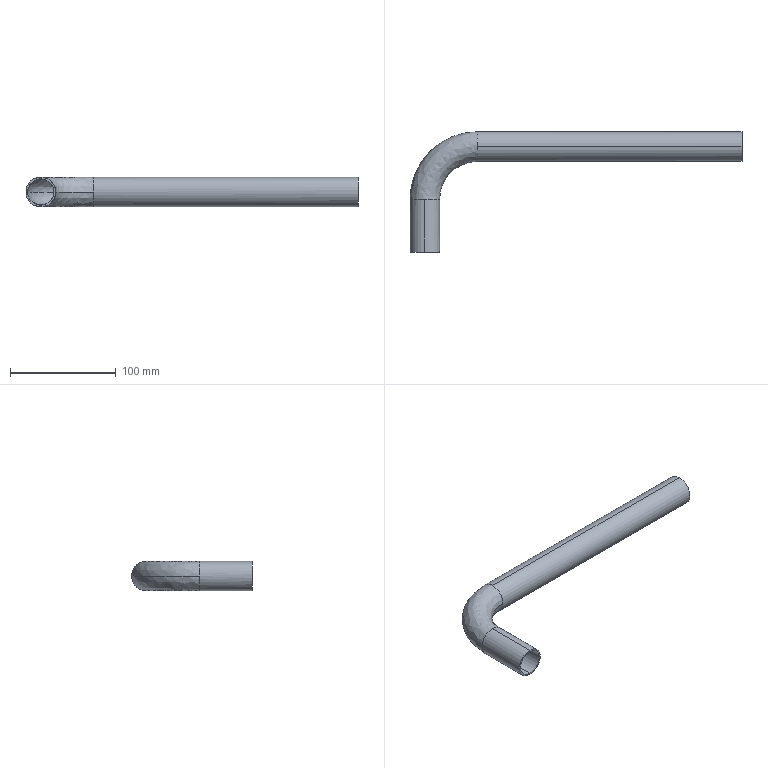Part | STEP file | copper tube 17_default_machined_ | 1 solid | 14 faces | box 314 x 114 x 28 mm | volume 47271 mm3 | cylinder 8 | spline 4 | plane 2 | commonest cylinder face diameters 25 x4 28 x4